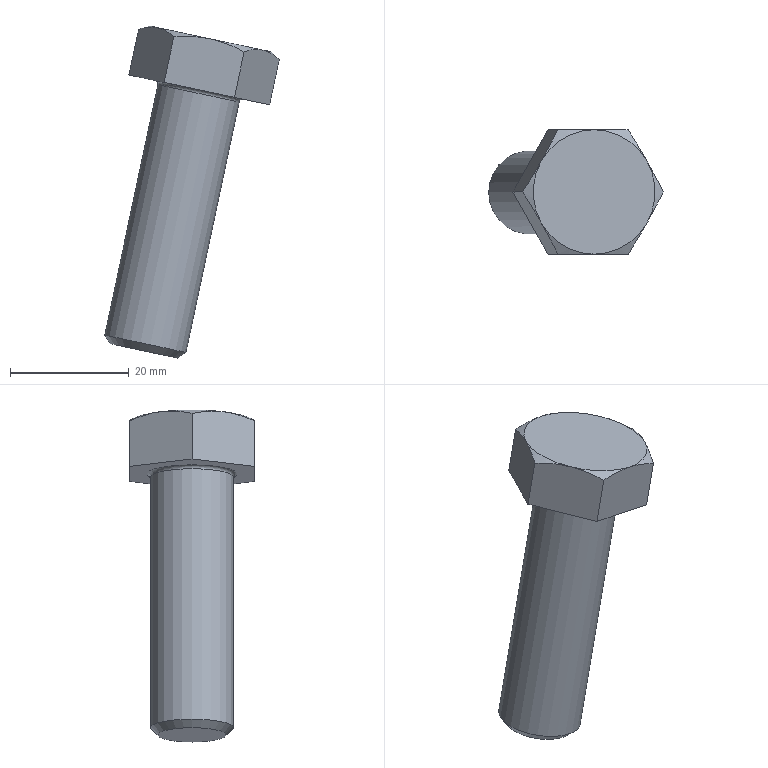Part | STEP file | 8901-M1445B bolt | 1 solid | 18 faces | box 29.442 x 21 x 56.008 mm | volume 10250 mm3 | plane 9 | cone 7 | cylinder 1 | torus 1 | commonest cylinder face diameters 14 x1